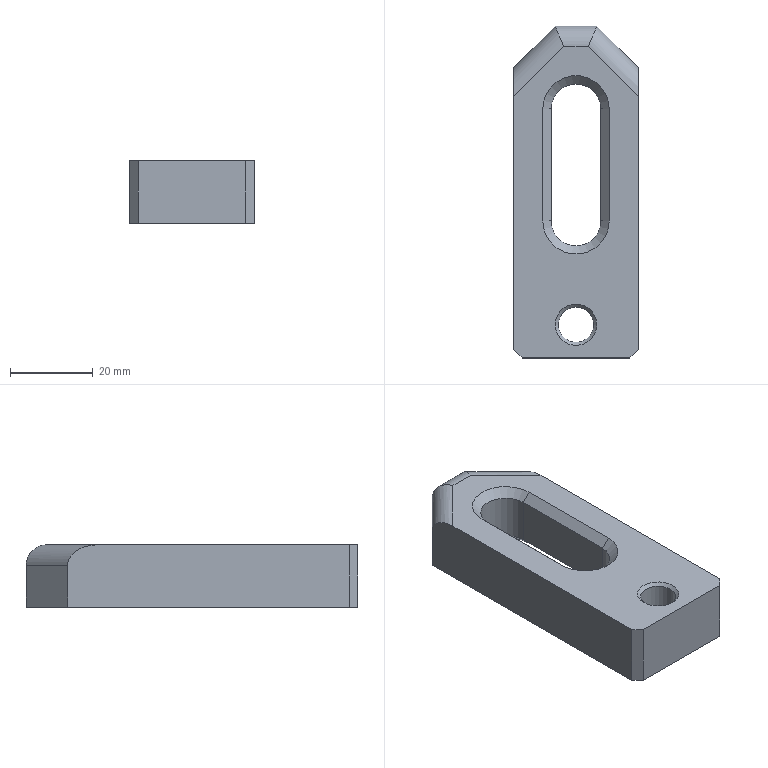Part | NX | features DATUM_CSYS 4, CHAMFER 3, SKETCH 3, EXTRUDE 2, BLEND 1, HOLE PACKAGE 1, SIMPLE HOLE 1, SYMBOLIC_THREAD 1 | 1 solid | 28 faces | box 30 x 80 x 15 mm | volume 26425 mm3 | plane 16 | cylinder 6 | cone 6 | commonest cylinder face diameters 10 x3 12 x2 8.5 x1
STEP:
#1=CARTESIAN_POINT('',(0.,70.,0.));
#2=VERTEX_POINT('',#1);
#3=CARTESIAN_POINT('',(0.,2.,0.));
#4=VERTEX_POINT('',#3);
#5=CARTESIAN_POINT('',(0.,80.,0.));
#6=DIRECTION('',(0.,-1.,0.));
#7=VECTOR('',#6,1000.);
#8=LINE('',#5,#7);
#9=EDGE_CURVE('',#2,#4,#8,.T.);
#10=ORIENTED_EDGE('',*,*,#9,.T.);
#11=CARTESIAN_POINT('',(0.,2.,15.));
#12=VERTEX_POINT('',#11);
#13=CARTESIAN_POINT('',(0.,2.,15.));
#14=DIRECTION('',(0.,0.,1.));
#15=VECTOR('',#14,1000.);
#16=LINE('',#13,#15);
#17=EDGE_CURVE('',#4,#12,#16,.T.);
#18=ORIENTED_EDGE('',*,*,#17,.T.);
#19=CARTESIAN_POINT('',(0.,62.929,15.));
#20=VERTEX_POINT('',#19);
#21=CARTESIAN_POINT('',(0.,80.,15.));
#22=DIRECTION('',(0.,-1.,0.));
#23=VECTOR('',#22,1000.);
#24=LINE('',#21,#23);
#25=EDGE_CURVE('',#20,#12,#24,.T.);
#26=ORIENTED_EDGE('',*,*,#25,.F.);
#27=CARTESIAN_POINT('',(0.,70.,10.));
#28=VERTEX_POINT('',#27);
#29=CARTESIAN_POINT('',(0.,62.929,10.));
#30=DIRECTION('',(1.,0.,0.));
#31=DIRECTION('',(0.,1.,0.));
#32=AXIS2_PLACEMENT_3D('',#29,#30,#31);
#33=ELLIPSE('',#32,7.071,5.);
#34=EDGE_CURVE('',#20,#28,#33,.F.);
#35=ORIENTED_EDGE('',*,*,#34,.T.);
#36=CARTESIAN_POINT('',(0.,70.,15.));
#37=DIRECTION('',(0.,0.,-1.));
#38=VECTOR('',#37,1000.);
#39=LINE('',#36,#38);
#40=EDGE_CURVE('',#28,#2,#39,.T.);
#41=ORIENTED_EDGE('',*,*,#40,.T.);
#42=EDGE_LOOP('',(#10,#18,#26,#35,#41));
#43=FACE_BOUND('',#42,.T.);
#44=CARTESIAN_POINT('',(0.,80.,15.));
#45=DIRECTION('',(1.,0.,0.));
#46=DIRECTION('',(0.,1.,0.));
#47=AXIS2_PLACEMENT_3D('',#44,#45,#46);
#48=PLANE('',#47);
#49=ADVANCED_FACE('',(#43),#48,.F.);
#50=CARTESIAN_POINT('',(2.,0.,15.));
#51=VERTEX_POINT('',#50);
#52=CARTESIAN_POINT('',(28.,0.,15.));
#53=VERTEX_POINT('',#52);
#54=CARTESIAN_POINT('',(0.,0.,15.));
#55=DIRECTION('',(1.,0.,0.));
#56=VECTOR('',#55,1000.);
#57=LINE('',#54,#56);
#58=EDGE_CURVE('',#51,#53,#57,.T.);
#59=ORIENTED_EDGE('',*,*,#58,.F.);
#60=CARTESIAN_POINT('',(2.,0.,0.));
#61=VERTEX_POINT('',#60);
#62=CARTESIAN_POINT('',(2.,0.,15.));
#63=DIRECTION('',(0.,0.,-1.));
#64=VECTOR('',#63,1000.);
#65=LINE('',#62,#64);
#66=EDGE_CURVE('',#51,#61,#65,.T.);
#67=ORIENTED_EDGE('',*,*,#66,.T.);
#68=CARTESIAN_POINT('',(28.,0.,0.));
#69=VERTEX_POINT('',#68);
#70=CARTESIAN_POINT('',(0.,0.,0.));
#71=DIRECTION('',(1.,0.,0.));
#72=VECTOR('',#71,1000.);
#73=LINE('',#70,#72);
#74=EDGE_CURVE('',#61,#69,#73,.T.);
#75=ORIENTED_EDGE('',*,*,#74,.T.);
#76=CARTESIAN_POINT('',(28.,0.,15.));
#77=DIRECTION('',(0.,0.,1.));
#78=VECTOR('',#77,1000.);
#79=LINE('',#76,#78);
#80=EDGE_CURVE('',#69,#53,#79,.T.);
#81=ORIENTED_EDGE('',*,*,#80,.T.);
#82=EDGE_LOOP('',(#59,#67,#75,#81));
#83=FACE_BOUND('',#82,.T.);
#84=CARTESIAN_POINT('',(0.,0.,15.));
#85=DIRECTION('',(0.,1.,0.));
#86=DIRECTION('',(0.,0.,1.));
#87=AXIS2_PLACEMENT_3D('',#84,#85,#86);
#88=PLANE('',#87);
#89=ADVANCED_FACE('',(#83),#88,.F.);
#90=CARTESIAN_POINT('',(30.,2.,15.));
#91=VERTEX_POINT('',#90);
#92=CARTESIAN_POINT('',(30.,62.929,15.));
#93=VERTEX_POINT('',#92);
#94=CARTESIAN_POINT('',(30.,0.,15.));
#95=DIRECTION('',(0.,1.,0.));
#96=VECTOR('',#95,1000.);
#97=LINE('',#94,#96);
#98=EDGE_CURVE('',#91,#93,#97,.T.);
#99=ORIENTED_EDGE('',*,*,#98,.F.);
#100=CARTESIAN_POINT('',(30.,2.,0.));
#101=VERTEX_POINT('',#100);
#102=CARTESIAN_POINT('',(30.,2.,15.));
#103=DIRECTION('',(0.,0.,-1.));
#104=VECTOR('',#103,1000.);
#105=LINE('',#102,#104);
#106=EDGE_CURVE('',#91,#101,#105,.T.);
#107=ORIENTED_EDGE('',*,*,#106,.T.);
#108=CARTESIAN_POINT('',(30.,70.,0.));
#109=VERTEX_POINT('',#108);
#110=CARTESIAN_POINT('',(30.,0.,0.));
#111=DIRECTION('',(0.,1.,0.));
#112=VECTOR('',#111,1000.);
#113=LINE('',#110,#112);
#114=EDGE_CURVE('',#101,#109,#113,.T.);
#115=ORIENTED_EDGE('',*,*,#114,.T.);
#116=CARTESIAN_POINT('',(30.,70.,10.));
#117=VERTEX_POINT('',#116);
#118=CARTESIAN_POINT('',(30.,70.,15.));
#119=DIRECTION('',(0.,0.,1.));
#120=VECTOR('',#119,1000.);
#121=LINE('',#118,#120);
#122=EDGE_CURVE('',#109,#117,#121,.T.);
#123=ORIENTED_EDGE('',*,*,#122,.T.);
#124=CARTESIAN_POINT('',(30.,62.929,10.));
#125=DIRECTION('',(-1.,0.,0.));
#126=DIRECTION('',(0.,-1.,0.));
#127=AXIS2_PLACEMENT_3D('',#124,#125,#126);
#128=ELLIPSE('',#127,7.071,5.);
#129=EDGE_CURVE('',#117,#93,#128,.F.);
#130=ORIENTED_EDGE('',*,*,#129,.T.);
#131=EDGE_LOOP('',(#99,#107,#115,#123,#130));
#132=FACE_BOUND('',#131,.T.);
#133=CARTESIAN_POINT('',(30.,0.,15.));
#134=DIRECTION('',(-1.,0.,0.));
#135=DIRECTION('',(0.,-1.,0.));
#136=AXIS2_PLACEMENT_3D('',#133,#134,#135);
#137=PLANE('',#136);
#138=ADVANCED_FACE('',(#132),#137,.F.);
#139=CARTESIAN_POINT('',(10.,80.,0.));
#140=VERTEX_POINT('',#139);
#141=CARTESIAN_POINT('',(10.,80.,10.));
#142=VERTEX_POINT('',#141);
#143=CARTESIAN_POINT('',(10.,80.,15.));
#144=DIRECTION('',(0.,0.,1.));
#145=VECTOR('',#144,1000.);
#146=LINE('',#143,#145);
#147=EDGE_CURVE('',#140,#142,#146,.T.);
#148=ORIENTED_EDGE('',*,*,#147,.T.);
#149=CARTESIAN_POINT('',(20.,80.,10.));
#150=VERTEX_POINT('',#149);
#151=CARTESIAN_POINT('',(20.,80.,10.));
#152=DIRECTION('',(-1.,0.,0.));
#153=VECTOR('',#152,1000.);
#154=LINE('',#151,#153);
#155=EDGE_CURVE('',#142,#150,#154,.F.);
#156=ORIENTED_EDGE('',*,*,#155,.T.);
#157=CARTESIAN_POINT('',(20.,80.,0.));
#158=VERTEX_POINT('',#157);
#159=CARTESIAN_POINT('',(20.,80.,15.));
#160=DIRECTION('',(0.,0.,-1.));
#161=VECTOR('',#160,1000.);
#162=LINE('',#159,#161);
#163=EDGE_CURVE('',#150,#158,#162,.T.);
#164=ORIENTED_EDGE('',*,*,#163,.T.);
#165=CARTESIAN_POINT('',(30.,80.,0.));
#166=DIRECTION('',(-1.,0.,0.));
#167=VECTOR('',#166,1000.);
#168=LINE('',#165,#167);
#169=EDGE_CURVE('',#158,#140,#168,.T.);
#170=ORIENTED_EDGE('',*,*,#169,.T.);
#171=EDGE_LOOP('',(#148,#156,#164,#170));
#172=FACE_BOUND('',#171,.T.);
#173=CARTESIAN_POINT('',(30.,80.,15.));
#174=DIRECTION('',(0.,-1.,0.));
#175=DIRECTION('',(0.,0.,-1.));
#176=AXIS2_PLACEMENT_3D('',#173,#174,#175);
#177=PLANE('',#176);
#178=ADVANCED_FACE('',(#172),#177,.F.);
#179=CARTESIAN_POINT('',(23.,60.,15.));
#180=VERTEX_POINT('',#179);
#181=CARTESIAN_POINT('',(23.,33.,15.));
#182=VERTEX_POINT('',#181);
#183=CARTESIAN_POINT('',(23.,33.,15.));
#184=DIRECTION('',(0.,-1.,0.));
#185=VECTOR('',#184,1000.);
#186=LINE('',#183,#185);
#187=EDGE_CURVE('',#180,#182,#186,.T.);
#188=ORIENTED_EDGE('',*,*,#187,.T.);
#189=CARTESIAN_POINT('',(7.,33.,15.));
#190=VERTEX_POINT('',#189);
#191=CARTESIAN_POINT('',(15.,33.,15.));
#192=DIRECTION('',(0.,0.,1.));
#193=DIRECTION('',(1.,0.,0.));
#194=AXIS2_PLACEMENT_3D('',#191,#192,#193);
#195=CIRCLE('',#194,8.);
#196=EDGE_CURVE('',#182,#190,#195,.F.);
#197=ORIENTED_EDGE('',*,*,#196,.T.);
#198=CARTESIAN_POINT('',(7.,60.,15.));
#199=VERTEX_POINT('',#198);
#200=CARTESIAN_POINT('',(7.,60.,15.));
#201=DIRECTION('',(0.,1.,0.));
#202=VECTOR('',#201,1000.);
#203=LINE('',#200,#202);
#204=EDGE_CURVE('',#190,#199,#203,.T.);
#205=ORIENTED_EDGE('',*,*,#204,.T.);
#206=CARTESIAN_POINT('',(15.,60.,15.));
#207=DIRECTION('',(0.,0.,1.));
#208=DIRECTION('',(1.,0.,0.));
#209=AXIS2_PLACEMENT_3D('',#206,#207,#208);
#210=CIRCLE('',#209,8.);
#211=EDGE_CURVE('',#199,#180,#210,.F.);
#212=ORIENTED_EDGE('',*,*,#211,.T.);
#213=EDGE_LOOP('',(#188,#197,#205,#212));
#214=FACE_BOUND('',#213,.T.);
#215=CARTESIAN_POINT('',(20.,8.,15.));
#216=VERTEX_POINT('',#215);
#217=CARTESIAN_POINT('',(15.,8.,15.));
#218=DIRECTION('',(0.,0.,1.));
#219=DIRECTION('',(1.,0.,0.));
#220=AXIS2_PLACEMENT_3D('',#217,#218,#219);
#221=CIRCLE('',#220,5.);
#222=EDGE_CURVE('',#216,#216,#221,.F.);
#223=ORIENTED_EDGE('',*,*,#222,.T.);
#224=EDGE_LOOP('',(#223));
#225=FACE_BOUND('',#224,.T.);
#226=ORIENTED_EDGE('',*,*,#25,.T.);
#227=CARTESIAN_POINT('',(1.,1.,15.));
#228=DIRECTION('',(-0.7071,0.7071,0.));
#229=VECTOR('',#228,1000.);
#230=LINE('',#227,#229);
#231=EDGE_CURVE('',#12,#51,#230,.F.);
#232=ORIENTED_EDGE('',*,*,#231,.T.);
#233=ORIENTED_EDGE('',*,*,#58,.T.);
#234=CARTESIAN_POINT('',(14.,-14.,15.));
#235=DIRECTION('',(-0.7071,-0.7071,0.));
#236=VECTOR('',#235,1000.);
#237=LINE('',#234,#236);
#238=EDGE_CURVE('',#53,#91,#237,.F.);
#239=ORIENTED_EDGE('',*,*,#238,.T.);
#240=ORIENTED_EDGE('',*,*,#98,.T.);
#241=CARTESIAN_POINT('',(17.929,75.,15.));
#242=VERTEX_POINT('',#241);
#243=CARTESIAN_POINT('',(46.464,46.464,15.));
#244=DIRECTION('',(0.7071,-0.7071,0.));
#245=VECTOR('',#244,1000.);
#246=LINE('',#243,#245);
#247=EDGE_CURVE('',#93,#242,#246,.F.);
#248=ORIENTED_EDGE('',*,*,#247,.T.);
#249=CARTESIAN_POINT('',(12.071,75.,15.));
#250=VERTEX_POINT('',#249);
#251=CARTESIAN_POINT('',(10.,75.,15.));
#252=DIRECTION('',(-1.,0.,0.));
#253=VECTOR('',#252,1000.);
#254=LINE('',#251,#253);
#255=EDGE_CURVE('',#242,#250,#254,.T.);
#256=ORIENTED_EDGE('',*,*,#255,.T.);
#257=CARTESIAN_POINT('',(-31.464,31.464,15.));
#258=DIRECTION('',(0.7071,0.7071,0.));
#259=VECTOR('',#258,1000.);
#260=LINE('',#257,#259);
#261=EDGE_CURVE('',#250,#20,#260,.F.);
#262=ORIENTED_EDGE('',*,*,#261,.T.);
#263=EDGE_LOOP('',(#226,#232,#233,#239,#240,#248,#256,#262));
#264=FACE_BOUND('',#263,.T.);
#265=CARTESIAN_POINT('',(0.,0.,15.));
#266=DIRECTION('',(0.,0.,1.));
#267=DIRECTION('',(1.,0.,0.));
#268=AXIS2_PLACEMENT_3D('',#265,#266,#267);
#269=PLANE('',#268);
#270=ADVANCED_FACE('',(#214,#225,#264),#269,.T.);
#271=CARTESIAN_POINT('',(7.,60.,0.));
#272=VERTEX_POINT('',#271);
#273=CARTESIAN_POINT('',(7.,33.,0.));
#274=VERTEX_POINT('',#273);
#275=CARTESIAN_POINT('',(7.,0.,0.));
#276=DIRECTION('',(0.,-1.,0.));
#277=VECTOR('',#276,1000.);
#278=LINE('',#275,#277);
#279=EDGE_CURVE('',#272,#274,#278,.T.);
#280=ORIENTED_EDGE('',*,*,#279,.T.);
#281=CARTESIAN_POINT('',(23.,33.,0.));
#282=VERTEX_POINT('',#281);
#283=CARTESIAN_POINT('',(15.,33.,0.));
#284=DIRECTION('',(0.,0.,1.));
#285=DIRECTION('',(1.,0.,0.));
#286=AXIS2_PLACEMENT_3D('',#283,#284,#285);
#287=CIRCLE('',#286,8.);
#288=EDGE_CURVE('',#274,#282,#287,.T.);
#289=ORIENTED_EDGE('',*,*,#288,.T.);
#290=CARTESIAN_POINT('',(23.,60.,0.));
#291=VERTEX_POINT('',#290);
#292=CARTESIAN_POINT('',(23.,0.,0.));
#293=DIRECTION('',(0.,1.,0.));
#294=VECTOR('',#293,1000.);
#295=LINE('',#292,#294);
#296=EDGE_CURVE('',#282,#291,#295,.T.);
#297=ORIENTED_EDGE('',*,*,#296,.T.);
#298=CARTESIAN_POINT('',(15.,60.,0.));
#299=DIRECTION('',(0.,0.,1.));
#300=DIRECTION('',(1.,0.,0.));
#301=AXIS2_PLACEMENT_3D('',#298,#299,#300);
#302=CIRCLE('',#301,8.);
#303=EDGE_CURVE('',#291,#272,#302,.T.);
#304=ORIENTED_EDGE('',*,*,#303,.T.);
#305=EDGE_LOOP('',(#280,#289,#297,#304));
#306=FACE_BOUND('',#305,.T.);
#307=CARTESIAN_POINT('',(20.,8.,0.));
#308=VERTEX_POINT('',#307);
#309=CARTESIAN_POINT('',(15.,8.,0.));
#310=DIRECTION('',(0.,0.,1.));
#311=DIRECTION('',(1.,0.,0.));
#312=AXIS2_PLACEMENT_3D('',#309,#310,#311);
#313=CIRCLE('',#312,5.);
#314=EDGE_CURVE('',#308,#308,#313,.T.);
#315=ORIENTED_EDGE('',*,*,#314,.T.);
#316=EDGE_LOOP('',(#315));
#317=FACE_BOUND('',#316,.T.);
#318=ORIENTED_EDGE('',*,*,#74,.F.);
#319=CARTESIAN_POINT('',(2.,0.,0.));
#320=DIRECTION('',(0.7071,-0.7071,0.));
#321=VECTOR('',#320,1000.);
#322=LINE('',#319,#321);
#323=EDGE_CURVE('',#61,#4,#322,.F.);
#324=ORIENTED_EDGE('',*,*,#323,.T.);
#325=ORIENTED_EDGE('',*,*,#9,.F.);
#326=CARTESIAN_POINT('',(0.,70.,0.));
#327=DIRECTION('',(-0.7071,-0.7071,0.));
#328=VECTOR('',#327,1000.);
#329=LINE('',#326,#328);
#330=EDGE_CURVE('',#2,#140,#329,.F.);
#331=ORIENTED_EDGE('',*,*,#330,.T.);
#332=ORIENTED_EDGE('',*,*,#169,.F.);
#333=CARTESIAN_POINT('',(20.,80.,0.));
#334=DIRECTION('',(-0.7071,0.7071,0.));
#335=VECTOR('',#334,1000.);
#336=LINE('',#333,#335);
#337=EDGE_CURVE('',#158,#109,#336,.F.);
#338=ORIENTED_EDGE('',*,*,#337,.T.);
#339=ORIENTED_EDGE('',*,*,#114,.F.);
#340=CARTESIAN_POINT('',(30.,2.,0.));
#341=DIRECTION('',(0.7071,0.7071,0.));
#342=VECTOR('',#341,1000.);
#343=LINE('',#340,#342);
#344=EDGE_CURVE('',#101,#69,#343,.F.);
#345=ORIENTED_EDGE('',*,*,#344,.T.);
#346=EDGE_LOOP('',(#318,#324,#325,#331,#332,#338,#339,#345));
#347=FACE_BOUND('',#346,.T.);
#348=CARTESIAN_POINT('',(0.,0.,0.));
#349=DIRECTION('',(0.,0.,1.));
#350=DIRECTION('',(1.,0.,0.));
#351=AXIS2_PLACEMENT_3D('',#348,#349,#350);
#352=PLANE('',#351);
#353=ADVANCED_FACE('',(#306,#317,#347),#352,.F.);
#354=ORIENTED_EDGE('',*,*,#163,.F.);
#355=CARTESIAN_POINT('',(20.,80.,10.));
#356=DIRECTION('',(-0.7071,0.7071,0.));
#357=VECTOR('',#356,1000.);
#358=LINE('',#355,#357);
#359=EDGE_CURVE('',#150,#117,#358,.F.);
#360=ORIENTED_EDGE('',*,*,#359,.T.);
#361=ORIENTED_EDGE('',*,*,#122,.F.);
#362=ORIENTED_EDGE('',*,*,#337,.F.);
#363=EDGE_LOOP('',(#354,#360,#361,#362));
#364=FACE_BOUND('',#363,.T.);
#365=CARTESIAN_POINT('',(20.,80.,15.));
#366=DIRECTION('',(-0.7071,-0.7071,0.));
#367=DIRECTION('',(0.,0.,-1.));
#368=AXIS2_PLACEMENT_3D('',#365,#366,#367);
#369=PLANE('',#368);
#370=ADVANCED_FACE('',(#364),#369,.F.);
#371=ORIENTED_EDGE('',*,*,#40,.F.);
#372=CARTESIAN_POINT('',(0.,70.,10.));
#373=DIRECTION('',(-0.7071,-0.7071,0.));
#374=VECTOR('',#373,1000.);
#375=LINE('',#372,#374);
#376=EDGE_CURVE('',#28,#142,#375,.F.);
#377=ORIENTED_EDGE('',*,*,#376,.T.);
#378=ORIENTED_EDGE('',*,*,#147,.F.);
#379=ORIENTED_EDGE('',*,*,#330,.F.);
#380=EDGE_LOOP('',(#371,#377,#378,#379));
#381=FACE_BOUND('',#380,.T.);
#382=CARTESIAN_POINT('',(0.,70.,15.));
#383=DIRECTION('',(0.7071,-0.7071,0.));
#384=DIRECTION('',(0.,0.,-1.));
#385=AXIS2_PLACEMENT_3D('',#382,#383,#384);
#386=PLANE('',#385);
#387=ADVANCED_FACE('',(#381),#386,.F.);
#388=CARTESIAN_POINT('',(9.,33.,13.));
#389=VERTEX_POINT('',#388);
#390=CARTESIAN_POINT('',(9.,33.,2.));
#391=VERTEX_POINT('',#390);
#392=CARTESIAN_POINT('',(9.,33.,-107.));
#393=DIRECTION('',(0.,0.,1.));
#394=VECTOR('',#393,1000.);
#395=LINE('',#392,#394);
#396=EDGE_CURVE('',#389,#391,#395,.F.);
#397=ORIENTED_EDGE('',*,*,#396,.T.);
#398=CARTESIAN_POINT('',(9.,60.,2.));
#399=VERTEX_POINT('',#398);
#400=CARTESIAN_POINT('',(9.,60.,2.));
#401=DIRECTION('',(0.,1.,0.));
#402=VECTOR('',#401,1000.);
#403=LINE('',#400,#402);
#404=EDGE_CURVE('',#391,#399,#403,.T.);
#405=ORIENTED_EDGE('',*,*,#404,.T.);
#406=CARTESIAN_POINT('',(9.,60.,13.));
#407=VERTEX_POINT('',#406);
#408=CARTESIAN_POINT('',(9.,60.,-107.));
#409=DIRECTION('',(0.,0.,1.));
#410=VECTOR('',#409,1000.);
#411=LINE('',#408,#410);
#412=EDGE_CURVE('',#407,#399,#411,.F.);
#413=ORIENTED_EDGE('',*,*,#412,.F.);
#414=CARTESIAN_POINT('',(9.,33.,13.));
#415=DIRECTION('',(0.,-1.,0.));
#416=VECTOR('',#415,1000.);
#417=LINE('',#414,#416);
#418=EDGE_CURVE('',#407,#389,#417,.T.);
#419=ORIENTED_EDGE('',*,*,#418,.T.);
#420=EDGE_LOOP('',(#397,#405,#413,#419));
#421=FACE_BOUND('',#420,.T.);
#422=CARTESIAN_POINT('',(9.,60.,-107.));
#423=DIRECTION('',(-1.,0.,0.));
#424=DIRECTION('',(0.,-1.,0.));
#425=AXIS2_PLACEMENT_3D('',#422,#423,#424);
#426=PLANE('',#425);
#427=ADVANCED_FACE('',(#421),#426,.F.);
#428=CARTESIAN_POINT('',(21.,33.,13.));
#429=VERTEX_POINT('',#428);
#430=CARTESIAN_POINT('',(21.,33.,2.));
#431=VERTEX_POINT('',#430);
#432=CARTESIAN_POINT('',(21.,33.,-107.));
#433=DIRECTION('',(0.,0.,1.));
#434=VECTOR('',#433,1000.);
#435=LINE('',#432,#434);
#436=EDGE_CURVE('',#429,#431,#435,.F.);
#437=ORIENTED_EDGE('',*,*,#436,.T.);
#438=CARTESIAN_POINT('',(15.,33.,2.));
#439=DIRECTION('',(0.,0.,1.));
#440=DIRECTION('',(1.,0.,0.));
#441=AXIS2_PLACEMENT_3D('',#438,#439,#440);
#442=CIRCLE('',#441,6.);
#443=EDGE_CURVE('',#431,#391,#442,.F.);
#444=ORIENTED_EDGE('',*,*,#443,.T.);
#445=ORIENTED_EDGE('',*,*,#396,.F.);
#446=CARTESIAN_POINT('',(15.,33.,13.));
#447=DIRECTION('',(0.,0.,1.));
#448=DIRECTION('',(1.,0.,0.));
#449=AXIS2_PLACEMENT_3D('',#446,#447,#448);
#450=CIRCLE('',#449,6.);
#451=EDGE_CURVE('',#389,#429,#450,.T.);
#452=ORIENTED_EDGE('',*,*,#451,.T.);
#453=EDGE_LOOP('',(#437,#444,#445,#452));
#454=FACE_BOUND('',#453,.T.);
#455=CARTESIAN_POINT('',(15.,33.,-107.));
#456=DIRECTION('',(0.,0.,1.));
#457=DIRECTION('',(1.,0.,0.));
#458=AXIS2_PLACEMENT_3D('',#455,#456,#457);
#459=CYLINDRICAL_SURFACE('',#458,6.);
#460=ADVANCED_FACE('',(#454),#459,.F.);
#461=CARTESIAN_POINT('',(21.,60.,13.));
#462=VERTEX_POINT('',#461);
#463=CARTESIAN_POINT('',(21.,60.,2.));
#464=VERTEX_POINT('',#463);
#465=CARTESIAN_POINT('',(21.,60.,-107.));
#466=DIRECTION('',(0.,0.,1.));
#467=VECTOR('',#466,1000.);
#468=LINE('',#465,#467);
#469=EDGE_CURVE('',#462,#464,#468,.F.);
#470=ORIENTED_EDGE('',*,*,#469,.T.);
#471=CARTESIAN_POINT('',(21.,33.,2.));
#472=DIRECTION('',(0.,-1.,0.));
#473=VECTOR('',#472,1000.);
#474=LINE('',#471,#473);
#475=EDGE_CURVE('',#464,#431,#474,.T.);
#476=ORIENTED_EDGE('',*,*,#475,.T.);
#477=ORIENTED_EDGE('',*,*,#436,.F.);
#478=CARTESIAN_POINT('',(21.,60.,13.));
#479=DIRECTION('',(0.,1.,0.));
#480=VECTOR('',#479,1000.);
#481=LINE('',#478,#480);
#482=EDGE_CURVE('',#429,#462,#481,.T.);
#483=ORIENTED_EDGE('',*,*,#482,.T.);
#484=EDGE_LOOP('',(#470,#476,#477,#483));
#485=FACE_BOUND('',#484,.T.);
#486=CARTESIAN_POINT('',(21.,33.,-107.));
#487=DIRECTION('',(1.,0.,0.));
#488=DIRECTION('',(0.,1.,0.));
#489=AXIS2_PLACEMENT_3D('',#486,#487,#488);
#490=PLANE('',#489);
#491=ADVANCED_FACE('',(#485),#490,.F.);
#492=ORIENTED_EDGE('',*,*,#412,.T.);
#493=CARTESIAN_POINT('',(15.,60.,2.));
#494=DIRECTION('',(0.,0.,1.));
#495=DIRECTION('',(1.,0.,0.));
#496=AXIS2_PLACEMENT_3D('',#493,#494,#495);
#497=CIRCLE('',#496,6.);
#498=EDGE_CURVE('',#399,#464,#497,.F.);
#499=ORIENTED_EDGE('',*,*,#498,.T.);
#500=ORIENTED_EDGE('',*,*,#469,.F.);
#501=CARTESIAN_POINT('',(15.,60.,13.));
#502=DIRECTION('',(0.,0.,1.));
#503=DIRECTION('',(1.,0.,0.));
#504=AXIS2_PLACEMENT_3D('',#501,#502,#503);
#505=CIRCLE('',#504,6.);
#506=EDGE_CURVE('',#462,#407,#505,.T.);
#507=ORIENTED_EDGE('',*,*,#506,.T.);
#508=EDGE_LOOP('',(#492,#499,#500,#507));
#509=FACE_BOUND('',#508,.T.);
#510=CARTESIAN_POINT('',(15.,60.,-107.));
#511=DIRECTION('',(0.,0.,1.));
#512=DIRECTION('',(1.,0.,0.));
#513=AXIS2_PLACEMENT_3D('',#510,#511,#512);
#514=CYLINDRICAL_SURFACE('',#513,6.);
#515=ADVANCED_FACE('',(#509),#514,.F.);
#516=CARTESIAN_POINT('',(19.25,8.,0.75));
#517=VERTEX_POINT('',#516);
#518=CARTESIAN_POINT('',(15.,8.,0.75));
#519=DIRECTION('',(0.,0.,1.));
#520=DIRECTION('',(1.,0.,0.));
#521=AXIS2_PLACEMENT_3D('',#518,#519,#520);
#522=CIRCLE('',#521,4.25);
#523=EDGE_CURVE('',#517,#517,#522,.F.);
#524=ORIENTED_EDGE('',*,*,#523,.T.);
#525=EDGE_LOOP('',(#524));
#526=FACE_BOUND('',#525,.T.);
#527=CARTESIAN_POINT('',(19.25,8.,14.25));
#528=VERTEX_POINT('',#527);
#529=CARTESIAN_POINT('',(15.,8.,14.25));
#530=DIRECTION('',(0.,0.,1.));
#531=DIRECTION('',(1.,0.,0.));
#532=AXIS2_PLACEMENT_3D('',#529,#530,#531);
#533=CIRCLE('',#532,4.25);
#534=EDGE_CURVE('',#528,#528,#533,.T.);
#535=ORIENTED_EDGE('',*,*,#534,.T.);
#536=EDGE_LOOP('',(#535));
#537=FACE_BOUND('',#536,.T.);
#538=CARTESIAN_POINT('',(15.,8.,15.));
#539=DIRECTION('',(0.,0.,-1.));
#540=DIRECTION('',(-1.,0.,0.));
#541=AXIS2_PLACEMENT_3D('',#538,#539,#540);
#542=CYLINDRICAL_SURFACE('',#541,4.25);
#543=ADVANCED_FACE('',(#526,#537),#542,.F.);
#544=ORIENTED_EDGE('',*,*,#534,.F.);
#545=EDGE_LOOP('',(#544));
#546=FACE_BOUND('',#545,.T.);
#547=ORIENTED_EDGE('',*,*,#222,.F.);
#548=EDGE_LOOP('',(#547));
#549=FACE_BOUND('',#548,.T.);
#550=CARTESIAN_POINT('',(15.,8.,15.));
#551=DIRECTION('',(0.,0.,1.));
#552=DIRECTION('',(1.,0.,0.));
#553=AXIS2_PLACEMENT_3D('',#550,#551,#552);
#554=CONICAL_SURFACE('',#553,5.,0.7854);
#555=ADVANCED_FACE('',(#546,#549),#554,.F.);
#556=ORIENTED_EDGE('',*,*,#523,.F.);
#557=EDGE_LOOP('',(#556));
#558=FACE_BOUND('',#557,.T.);
#559=ORIENTED_EDGE('',*,*,#314,.F.);
#560=EDGE_LOOP('',(#559));
#561=FACE_BOUND('',#560,.T.);
#562=CARTESIAN_POINT('',(15.,8.,0.));
#563=DIRECTION('',(0.,0.,-1.));
#564=DIRECTION('',(-1.,0.,0.));
#565=AXIS2_PLACEMENT_3D('',#562,#563,#564);
#566=CONICAL_SURFACE('',#565,5.,0.7854);
#567=ADVANCED_FACE('',(#558,#561),#566,.F.);
#568=CARTESIAN_POINT('',(21.,60.,2.));
#569=DIRECTION('',(0.7071,0.,-0.7071));
#570=VECTOR('',#569,1000.);
#571=LINE('',#568,#570);
#572=EDGE_CURVE('',#464,#291,#571,.T.);
#573=ORIENTED_EDGE('',*,*,#572,.F.);
#574=ORIENTED_EDGE('',*,*,#498,.F.);
#575=CARTESIAN_POINT('',(7.,60.,0.));
#576=DIRECTION('',(0.7071,0.,0.7071));
#577=VECTOR('',#576,1000.);
#578=LINE('',#575,#577);
#579=EDGE_CURVE('',#272,#399,#578,.T.);
#580=ORIENTED_EDGE('',*,*,#579,.F.);
#581=ORIENTED_EDGE('',*,*,#303,.F.);
#582=EDGE_LOOP('',(#573,#574,#580,#581));
#583=FACE_BOUND('',#582,.T.);
#584=CARTESIAN_POINT('',(15.,60.,0.));
#585=DIRECTION('',(0.,0.,-1.));
#586=DIRECTION('',(-1.,0.,0.));
#587=AXIS2_PLACEMENT_3D('',#584,#585,#586);
#588=CONICAL_SURFACE('',#587,8.,0.7854);
#589=ADVANCED_FACE('',(#583),#588,.F.);
#590=ORIENTED_EDGE('',*,*,#579,.T.);
#591=ORIENTED_EDGE('',*,*,#404,.F.);
#592=CARTESIAN_POINT('',(7.,33.,0.));
#593=DIRECTION('',(0.7071,0.,0.7071));
#594=VECTOR('',#593,1000.);
#595=LINE('',#592,#594);
#596=EDGE_CURVE('',#274,#391,#595,.T.);
#597=ORIENTED_EDGE('',*,*,#596,.F.);
#598=ORIENTED_EDGE('',*,*,#279,.F.);
#599=EDGE_LOOP('',(#590,#591,#597,#598));
#600=FACE_BOUND('',#599,.T.);
#601=CARTESIAN_POINT('',(7.,0.,0.));
#602=DIRECTION('',(-0.7071,0.,0.7071));
#603=DIRECTION('',(0.,-1.,0.));
#604=AXIS2_PLACEMENT_3D('',#601,#602,#603);
#605=PLANE('',#604);
#606=ADVANCED_FACE('',(#600),#605,.F.);
#607=ORIENTED_EDGE('',*,*,#572,.T.);
#608=ORIENTED_EDGE('',*,*,#296,.F.);
#609=CARTESIAN_POINT('',(21.,33.,2.));
#610=DIRECTION('',(0.7071,0.,-0.7071));
#611=VECTOR('',#610,1000.);
#612=LINE('',#609,#611);
#613=EDGE_CURVE('',#431,#282,#612,.T.);
#614=ORIENTED_EDGE('',*,*,#613,.F.);
#615=ORIENTED_EDGE('',*,*,#475,.F.);
#616=EDGE_LOOP('',(#607,#608,#614,#615));
#617=FACE_BOUND('',#616,.T.);
#618=CARTESIAN_POINT('',(23.,0.,0.));
#619=DIRECTION('',(0.7071,0.,0.7071));
#620=DIRECTION('',(0.,1.,0.));
#621=AXIS2_PLACEMENT_3D('',#618,#619,#620);
#622=PLANE('',#621);
#623=ADVANCED_FACE('',(#617),#622,.F.);
#624=ORIENTED_EDGE('',*,*,#596,.T.);
#625=ORIENTED_EDGE('',*,*,#443,.F.);
#626=ORIENTED_EDGE('',*,*,#613,.T.);
#627=ORIENTED_EDGE('',*,*,#288,.F.);
#628=EDGE_LOOP('',(#624,#625,#626,#627));
#629=FACE_BOUND('',#628,.T.);
#630=CARTESIAN_POINT('',(15.,33.,0.));
#631=DIRECTION('',(0.,0.,-1.));
#632=DIRECTION('',(-1.,0.,0.));
#633=AXIS2_PLACEMENT_3D('',#630,#631,#632);
#634=CONICAL_SURFACE('',#633,8.,0.7854);
#635=ADVANCED_FACE('',(#629),#634,.F.);
#636=CARTESIAN_POINT('',(23.,60.,15.));
#637=DIRECTION('',(-0.7071,0.,-0.7071));
#638=VECTOR('',#637,1000.);
#639=LINE('',#636,#638);
#640=EDGE_CURVE('',#180,#462,#639,.T.);
#641=ORIENTED_EDGE('',*,*,#640,.F.);
#642=ORIENTED_EDGE('',*,*,#211,.F.);
#643=CARTESIAN_POINT('',(9.,60.,13.));
#644=DIRECTION('',(-0.7071,0.,0.7071));
#645=VECTOR('',#644,1000.);
#646=LINE('',#643,#645);
#647=EDGE_CURVE('',#407,#199,#646,.T.);
#648=ORIENTED_EDGE('',*,*,#647,.F.);
#649=ORIENTED_EDGE('',*,*,#506,.F.);
#650=EDGE_LOOP('',(#641,#642,#648,#649));
#651=FACE_BOUND('',#650,.T.);
#652=CARTESIAN_POINT('',(15.,60.,13.));
#653=DIRECTION('',(0.,0.,1.));
#654=DIRECTION('',(1.,0.,0.));
#655=AXIS2_PLACEMENT_3D('',#652,#653,#654);
#656=CONICAL_SURFACE('',#655,6.,0.7854);
#657=ADVANCED_FACE('',(#651),#656,.F.);
#658=ORIENTED_EDGE('',*,*,#647,.T.);
#659=ORIENTED_EDGE('',*,*,#204,.F.);
#660=CARTESIAN_POINT('',(9.,33.,13.));
#661=DIRECTION('',(-0.7071,0.,0.7071));
#662=VECTOR('',#661,1000.);
#663=LINE('',#660,#662);
#664=EDGE_CURVE('',#389,#190,#663,.T.);
#665=ORIENTED_EDGE('',*,*,#664,.F.);
#666=ORIENTED_EDGE('',*,*,#418,.F.);
#667=EDGE_LOOP('',(#658,#659,#665,#666));
#668=FACE_BOUND('',#667,.T.);
#669=CARTESIAN_POINT('',(9.,60.,13.));
#670=DIRECTION('',(0.7071,0.,0.7071));
#671=DIRECTION('',(0.,1.,0.));
#672=AXIS2_PLACEMENT_3D('',#669,#670,#671);
#673=PLANE('',#672);
#674=ADVANCED_FACE('',(#668),#673,.T.);
#675=ORIENTED_EDGE('',*,*,#640,.T.);
#676=ORIENTED_EDGE('',*,*,#482,.F.);
#677=CARTESIAN_POINT('',(23.,33.,15.));
#678=DIRECTION('',(-0.7071,0.,-0.7071));
#679=VECTOR('',#678,1000.);
#680=LINE('',#677,#679);
#681=EDGE_CURVE('',#182,#429,#680,.T.);
#682=ORIENTED_EDGE('',*,*,#681,.F.);
#683=ORIENTED_EDGE('',*,*,#187,.F.);
#684=EDGE_LOOP('',(#675,#676,#682,#683));
#685=FACE_BOUND('',#684,.T.);
#686=CARTESIAN_POINT('',(21.,33.,13.));
#687=DIRECTION('',(-0.7071,0.,0.7071));
#688=DIRECTION('',(0.,-1.,0.));
#689=AXIS2_PLACEMENT_3D('',#686,#687,#688);
#690=PLANE('',#689);
#691=ADVANCED_FACE('',(#685),#690,.T.);
#692=ORIENTED_EDGE('',*,*,#664,.T.);
#693=ORIENTED_EDGE('',*,*,#196,.F.);
#694=ORIENTED_EDGE('',*,*,#681,.T.);
#695=ORIENTED_EDGE('',*,*,#451,.F.);
#696=EDGE_LOOP('',(#692,#693,#694,#695));
#697=FACE_BOUND('',#696,.T.);
#698=CARTESIAN_POINT('',(15.,33.,13.));
#699=DIRECTION('',(0.,0.,1.));
#700=DIRECTION('',(1.,0.,0.));
#701=AXIS2_PLACEMENT_3D('',#698,#699,#700);
#702=CONICAL_SURFACE('',#701,6.,0.7854);
#703=ADVANCED_FACE('',(#697),#702,.F.);
#704=ORIENTED_EDGE('',*,*,#129,.F.);
#705=ORIENTED_EDGE('',*,*,#359,.F.);
#706=CARTESIAN_POINT('',(17.929,75.,10.));
#707=DIRECTION('',(0.9239,-0.3827,0.));
#708=DIRECTION('',(0.3827,0.9239,0.));
#709=AXIS2_PLACEMENT_3D('',#706,#707,#708);
#710=ELLIPSE('',#709,5.412,5.);
#711=EDGE_CURVE('',#242,#150,#710,.F.);
#712=ORIENTED_EDGE('',*,*,#711,.F.);
#713=ORIENTED_EDGE('',*,*,#247,.F.);
#714=EDGE_LOOP('',(#704,#705,#712,#713));
#715=FACE_BOUND('',#714,.T.);
#716=CARTESIAN_POINT('',(46.464,46.464,10.));
#717=DIRECTION('',(0.7071,-0.7071,0.));
#718=DIRECTION('',(0.7071,0.7071,0.));
#719=AXIS2_PLACEMENT_3D('',#716,#717,#718);
#720=CYLINDRICAL_SURFACE('',#719,5.);
#721=ADVANCED_FACE('',(#715),#720,.T.);
#722=ORIENTED_EDGE('',*,*,#711,.T.);
#723=ORIENTED_EDGE('',*,*,#155,.F.);
#724=CARTESIAN_POINT('',(12.071,75.,10.));
#725=DIRECTION('',(0.9239,0.3827,0.));
#726=DIRECTION('',(0.3827,-0.9239,0.));
#727=AXIS2_PLACEMENT_3D('',#724,#725,#726);
#728=ELLIPSE('',#727,5.412,5.);
#729=EDGE_CURVE('',#250,#142,#728,.F.);
#730=ORIENTED_EDGE('',*,*,#729,.F.);
#731=ORIENTED_EDGE('',*,*,#255,.F.);
#732=EDGE_LOOP('',(#722,#723,#730,#731));
#733=FACE_BOUND('',#732,.T.);
#734=CARTESIAN_POINT('',(0.,75.,10.));
#735=DIRECTION('',(1.,0.,0.));
#736=DIRECTION('',(0.,0.,-1.));
#737=AXIS2_PLACEMENT_3D('',#734,#735,#736);
#738=CYLINDRICAL_SURFACE('',#737,5.);
#739=ADVANCED_FACE('',(#733),#738,.T.);
#740=ORIENTED_EDGE('',*,*,#729,.T.);
#741=ORIENTED_EDGE('',*,*,#376,.F.);
#742=ORIENTED_EDGE('',*,*,#34,.F.);
#743=ORIENTED_EDGE('',*,*,#261,.F.);
#744=EDGE_LOOP('',(#740,#741,#742,#743));
#745=FACE_BOUND('',#744,.T.);
#746=CARTESIAN_POINT('',(-31.464,31.464,10.));
#747=DIRECTION('',(0.7071,0.7071,0.));
#748=DIRECTION('',(-0.7071,0.7071,0.));
#749=AXIS2_PLACEMENT_3D('',#746,#747,#748);
#750=CYLINDRICAL_SURFACE('',#749,5.);
#751=ADVANCED_FACE('',(#745),#750,.T.);
#752=ORIENTED_EDGE('',*,*,#231,.F.);
#753=ORIENTED_EDGE('',*,*,#17,.F.);
#754=ORIENTED_EDGE('',*,*,#323,.F.);
#755=ORIENTED_EDGE('',*,*,#66,.F.);
#756=EDGE_LOOP('',(#752,#753,#754,#755));
#757=FACE_BOUND('',#756,.T.);
#758=CARTESIAN_POINT('',(2.,0.,15.));
#759=DIRECTION('',(0.7071,0.7071,0.));
#760=DIRECTION('',(0.,0.,-1.));
#761=AXIS2_PLACEMENT_3D('',#758,#759,#760);
#762=PLANE('',#761);
#763=ADVANCED_FACE('',(#757),#762,.F.);
#764=ORIENTED_EDGE('',*,*,#238,.F.);
#765=ORIENTED_EDGE('',*,*,#80,.F.);
#766=ORIENTED_EDGE('',*,*,#344,.F.);
#767=ORIENTED_EDGE('',*,*,#106,.F.);
#768=EDGE_LOOP('',(#764,#765,#766,#767));
#769=FACE_BOUND('',#768,.T.);
#770=CARTESIAN_POINT('',(30.,2.,15.));
#771=DIRECTION('',(-0.7071,0.7071,0.));
#772=DIRECTION('',(0.,0.,-1.));
#773=AXIS2_PLACEMENT_3D('',#770,#771,#772);
#774=PLANE('',#773);
#775=ADVANCED_FACE('',(#769),#774,.F.);
#776=CLOSED_SHELL('',(#49,#89,#138,#178,#270,#353,#370,#387,#427,#460,#491,#515,#543,#555,#567,#589,#606,#623,#635,#657,#674,#691,#703,#721,#739,#751,#763,#775));
#777=MANIFOLD_SOLID_BREP('',#776);
#778=(LENGTH_UNIT()NAMED_UNIT(*)SI_UNIT(.MILLI.,.METRE.));
#779=UNCERTAINTY_MEASURE_WITH_UNIT(LENGTH_MEASURE(0.00001),#778,'','');
#780=(NAMED_UNIT(*)PLANE_ANGLE_UNIT()SI_UNIT($,.RADIAN.));
#781=(NAMED_UNIT(*)SI_UNIT($,.STERADIAN.)SOLID_ANGLE_UNIT());
#782=(GEOMETRIC_REPRESENTATION_CONTEXT(3)GLOBAL_UNCERTAINTY_ASSIGNED_CONTEXT((#779))GLOBAL_UNIT_ASSIGNED_CONTEXT((#778,#780,#781))REPRESENTATION_CONTEXT('',''));
#783=ADVANCED_BREP_SHAPE_REPRESENTATION('',(#777),#782);